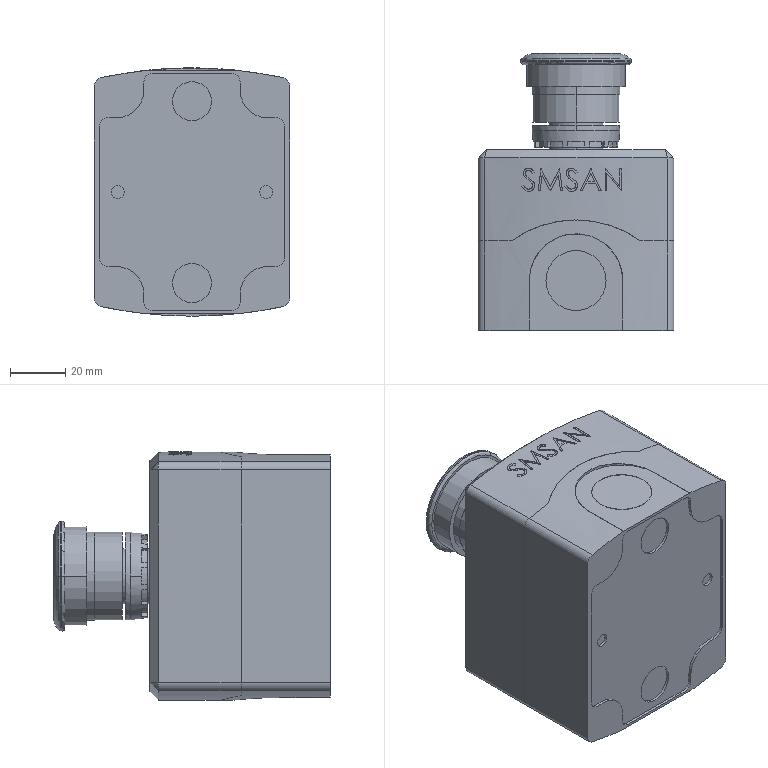Part | NX | features BREP 13 | 13 solids | 1035 faces | box 71 x 100.5 x 90.1 mm | volume 166359 mm3 | plane 545 | cylinder 306 | spline 64 | torus 63 | sphere 44 | cone 13 | commonest cylinder face diameters 0.2 x92 0.6 x24 0.4 x20 2 x18 6 x18 27.8 x13